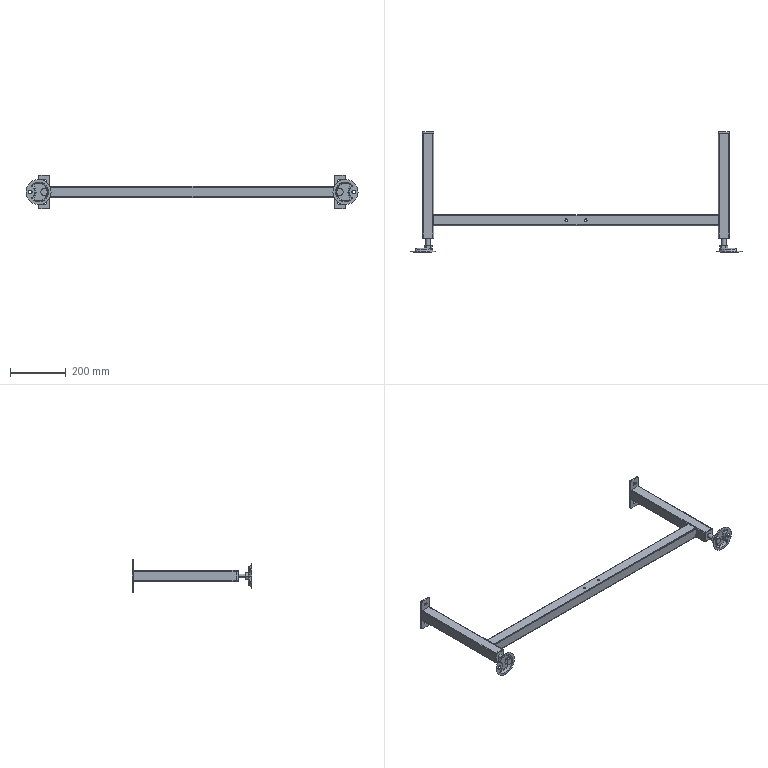Part | SolidWorks | 9 solids | 284 faces | box 1190 x 430 x 120 mm | volume 533595 mm3 | plane 116 | cylinder 92 | cone 40 | sphere 16 | torus 12 | spline 8 | commonest cylinder face diameters 6 x20 9 x16 2 x12 3 x12 10 x8 14 x8